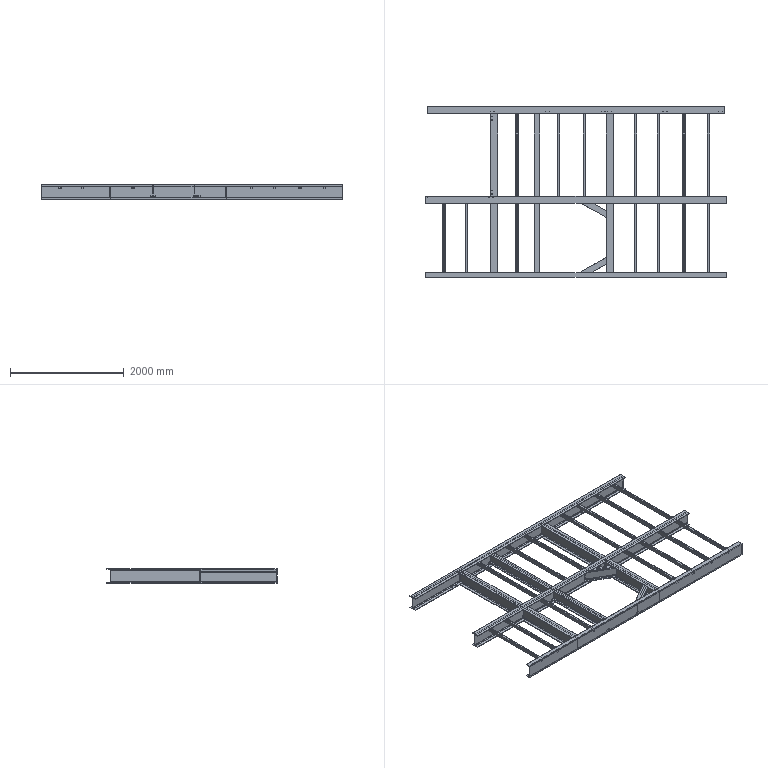Part | STEP file | PN_0042 second-floor transition bin platform deck_Default<As Machined> | 25 solids | 714 faces | box 5275 x 2990 x 250 mm | volume 103147929 mm3 | plane 489 | cylinder 224 | cone 1 | commonest cylinder face diameters 12 x78 6 x56 26 x40 24 x22 6.8 x20 18 x8